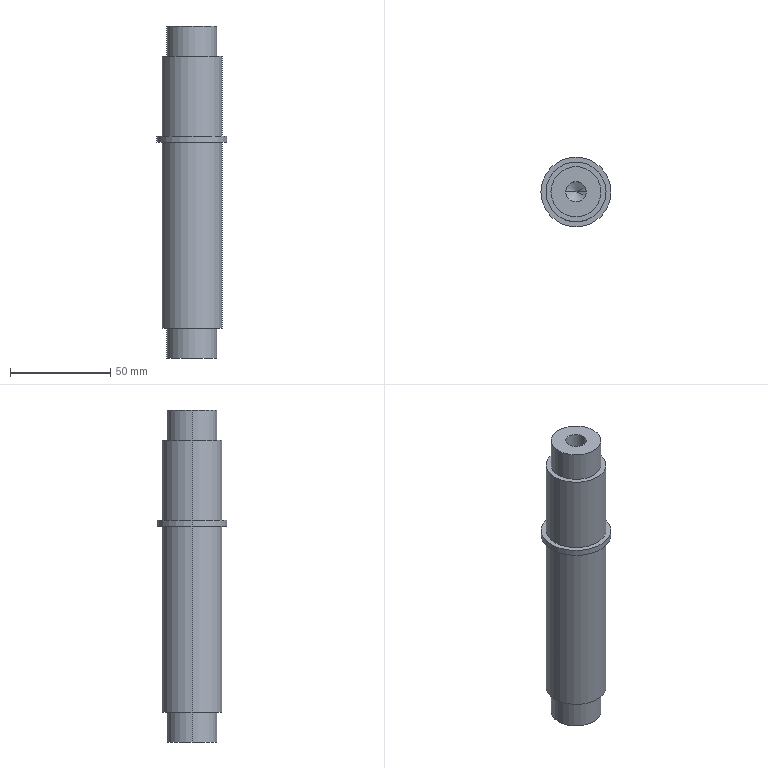Part | SolidWorks | features HoleWzd 2, ICE 2, Extrusion 1, MirrorPattern 1 | 1 solid | 24 faces | box 35 x 35 x 166 mm | volume 106106 mm3 | cylinder 14 | plane 6 | cone 4 | commonest cylinder face diameters 10.2 x4 25 x4 30 x4 35 x2
STEP:
#1=CARTESIAN_POINT('',(-5.1,0.,50.25));
#2=VERTEX_POINT('',#1);
#3=CARTESIAN_POINT('',(5.1,0.,50.25));
#4=VERTEX_POINT('',#3);
#5=CARTESIAN_POINT('',(0.,0.,50.25));
#6=DIRECTION('',(0.,0.,1.));
#7=DIRECTION('',(1.,0.,0.));
#8=AXIS2_PLACEMENT_3D('',#5,#6,#7);
#9=CIRCLE('',#8,5.1);
#10=EDGE_CURVE('',#2,#4,#9,.T.);
#11=ORIENTED_EDGE('',*,*,#10,.F.);
#12=CARTESIAN_POINT('',(-5.1,0.,83.));
#13=VERTEX_POINT('',#12);
#14=CARTESIAN_POINT('',(-5.1,0.,83.));
#15=DIRECTION('',(0.,0.,1.));
#16=VECTOR('',#15,1000.);
#17=LINE('',#14,#16);
#18=EDGE_CURVE('',#2,#13,#17,.T.);
#19=ORIENTED_EDGE('',*,*,#18,.T.);
#20=CARTESIAN_POINT('',(5.1,0.,83.));
#21=VERTEX_POINT('',#20);
#22=CARTESIAN_POINT('',(0.,0.,83.));
#23=DIRECTION('',(0.,0.,1.));
#24=DIRECTION('',(1.,0.,0.));
#25=AXIS2_PLACEMENT_3D('',#22,#23,#24);
#26=CIRCLE('',#25,5.1);
#27=EDGE_CURVE('',#13,#21,#26,.T.);
#28=ORIENTED_EDGE('',*,*,#27,.T.);
#29=CARTESIAN_POINT('',(5.1,0.,83.));
#30=DIRECTION('',(0.,0.,1.));
#31=VECTOR('',#30,1000.);
#32=LINE('',#29,#31);
#33=EDGE_CURVE('',#4,#21,#32,.T.);
#34=ORIENTED_EDGE('',*,*,#33,.F.);
#35=EDGE_LOOP('',(#11,#19,#28,#34));
#36=FACE_OUTER_BOUND('',#35,.T.);
#37=CARTESIAN_POINT('',(0.,0.,83.));
#38=DIRECTION('',(0.,0.,1.));
#39=DIRECTION('',(1.,0.,0.));
#40=AXIS2_PLACEMENT_3D('',#37,#38,#39);
#41=CYLINDRICAL_SURFACE('',#40,5.1);
#42=ADVANCED_FACE('',(#36),#41,.F.);
#43=CARTESIAN_POINT('',(0.,0.,47.186));
#44=VERTEX_POINT('',#43);
#45=CARTESIAN_POINT('',(5.1,0.,50.25));
#46=DIRECTION('',(0.8572,0.,0.515));
#47=VECTOR('',#46,1000.);
#48=LINE('',#45,#47);
#49=EDGE_CURVE('',#44,#4,#48,.T.);
#50=ORIENTED_EDGE('',*,*,#49,.F.);
#51=CARTESIAN_POINT('',(-5.1,0.,50.25));
#52=DIRECTION('',(-0.8572,0.,0.515));
#53=VECTOR('',#52,1000.);
#54=LINE('',#51,#53);
#55=EDGE_CURVE('',#44,#2,#54,.T.);
#56=ORIENTED_EDGE('',*,*,#55,.T.);
#57=ORIENTED_EDGE('',*,*,#10,.T.);
#58=EDGE_LOOP('',(#50,#56,#57));
#59=FACE_OUTER_BOUND('',#58,.T.);
#60=CARTESIAN_POINT('',(0.,0.,50.25));
#61=DIRECTION('',(0.,0.,1.));
#62=DIRECTION('',(1.,0.,0.));
#63=AXIS2_PLACEMENT_3D('',#60,#61,#62);
#64=CONICAL_SURFACE('',#63,5.1,1.03);
#65=ADVANCED_FACE('',(#59),#64,.F.);
#66=CARTESIAN_POINT('',(5.1,0.,-50.25));
#67=VERTEX_POINT('',#66);
#68=CARTESIAN_POINT('',(-5.1,0.,-50.25));
#69=VERTEX_POINT('',#68);
#70=CARTESIAN_POINT('',(0.,0.,-50.25));
#71=DIRECTION('',(0.,0.,-1.));
#72=DIRECTION('',(-1.,0.,0.));
#73=AXIS2_PLACEMENT_3D('',#70,#71,#72);
#74=CIRCLE('',#73,5.1);
#75=EDGE_CURVE('',#67,#69,#74,.T.);
#76=ORIENTED_EDGE('',*,*,#75,.F.);
#77=CARTESIAN_POINT('',(5.1,0.,-83.));
#78=VERTEX_POINT('',#77);
#79=CARTESIAN_POINT('',(5.1,0.,-83.));
#80=DIRECTION('',(0.,0.,-1.));
#81=VECTOR('',#80,1000.);
#82=LINE('',#79,#81);
#83=EDGE_CURVE('',#67,#78,#82,.T.);
#84=ORIENTED_EDGE('',*,*,#83,.T.);
#85=CARTESIAN_POINT('',(-5.1,0.,-83.));
#86=VERTEX_POINT('',#85);
#87=CARTESIAN_POINT('',(0.,0.,-83.));
#88=DIRECTION('',(0.,0.,-1.));
#89=DIRECTION('',(-1.,0.,0.));
#90=AXIS2_PLACEMENT_3D('',#87,#88,#89);
#91=CIRCLE('',#90,5.1);
#92=EDGE_CURVE('',#78,#86,#91,.T.);
#93=ORIENTED_EDGE('',*,*,#92,.T.);
#94=CARTESIAN_POINT('',(-5.1,0.,-83.));
#95=DIRECTION('',(0.,0.,-1.));
#96=VECTOR('',#95,1000.);
#97=LINE('',#94,#96);
#98=EDGE_CURVE('',#69,#86,#97,.T.);
#99=ORIENTED_EDGE('',*,*,#98,.F.);
#100=EDGE_LOOP('',(#76,#84,#93,#99));
#101=FACE_OUTER_BOUND('',#100,.T.);
#102=CARTESIAN_POINT('',(0.,0.,-83.));
#103=DIRECTION('',(0.,0.,-1.));
#104=DIRECTION('',(-1.,0.,0.));
#105=AXIS2_PLACEMENT_3D('',#102,#103,#104);
#106=CYLINDRICAL_SURFACE('',#105,5.1);
#107=ADVANCED_FACE('',(#101),#106,.F.);
#108=CARTESIAN_POINT('',(0.,0.,-47.186));
#109=VERTEX_POINT('',#108);
#110=CARTESIAN_POINT('',(-5.1,0.,-50.25));
#111=DIRECTION('',(-0.8572,0.,-0.515));
#112=VECTOR('',#111,1000.);
#113=LINE('',#110,#112);
#114=EDGE_CURVE('',#109,#69,#113,.T.);
#115=ORIENTED_EDGE('',*,*,#114,.F.);
#116=CARTESIAN_POINT('',(5.1,0.,-50.25));
#117=DIRECTION('',(0.8572,0.,-0.515));
#118=VECTOR('',#117,1000.);
#119=LINE('',#116,#118);
#120=EDGE_CURVE('',#109,#67,#119,.T.);
#121=ORIENTED_EDGE('',*,*,#120,.T.);
#122=ORIENTED_EDGE('',*,*,#75,.T.);
#123=EDGE_LOOP('',(#115,#121,#122));
#124=FACE_OUTER_BOUND('',#123,.T.);
#125=CARTESIAN_POINT('',(0.,0.,-50.25));
#126=DIRECTION('',(0.,0.,-1.));
#127=DIRECTION('',(-1.,0.,0.));
#128=AXIS2_PLACEMENT_3D('',#125,#126,#127);
#129=CONICAL_SURFACE('',#128,5.1,1.03);
#130=ADVANCED_FACE('',(#124),#129,.F.);
#131=CARTESIAN_POINT('',(15.,0.,25.));
#132=VERTEX_POINT('',#131);
#133=CARTESIAN_POINT('',(-15.,0.,25.));
#134=VERTEX_POINT('',#133);
#135=CARTESIAN_POINT('',(0.,0.,25.));
#136=DIRECTION('',(0.,0.,1.));
#137=DIRECTION('',(1.,0.,0.));
#138=AXIS2_PLACEMENT_3D('',#135,#136,#137);
#139=CIRCLE('',#138,15.);
#140=EDGE_CURVE('',#132,#134,#139,.T.);
#141=ORIENTED_EDGE('',*,*,#140,.F.);
#142=CARTESIAN_POINT('',(15.,0.,-68.));
#143=VERTEX_POINT('',#142);
#144=CARTESIAN_POINT('',(15.,0.,68.));
#145=DIRECTION('',(0.,0.,-1.));
#146=VECTOR('',#145,1000.);
#147=LINE('',#144,#146);
#148=EDGE_CURVE('',#132,#143,#147,.T.);
#149=ORIENTED_EDGE('',*,*,#148,.T.);
#150=CARTESIAN_POINT('',(-15.,0.,-68.));
#151=VERTEX_POINT('',#150);
#152=CARTESIAN_POINT('',(0.,0.,-68.));
#153=DIRECTION('',(0.,0.,1.));
#154=DIRECTION('',(1.,0.,0.));
#155=AXIS2_PLACEMENT_3D('',#152,#153,#154);
#156=CIRCLE('',#155,15.);
#157=EDGE_CURVE('',#143,#151,#156,.T.);
#158=ORIENTED_EDGE('',*,*,#157,.T.);
#159=CARTESIAN_POINT('',(-15.,0.,68.));
#160=DIRECTION('',(0.,0.,-1.));
#161=VECTOR('',#160,1000.);
#162=LINE('',#159,#161);
#163=EDGE_CURVE('',#134,#151,#162,.T.);
#164=ORIENTED_EDGE('',*,*,#163,.F.);
#165=EDGE_LOOP('',(#141,#149,#158,#164));
#166=FACE_OUTER_BOUND('',#165,.T.);
#167=CARTESIAN_POINT('',(0.,0.,68.));
#168=DIRECTION('',(0.,0.,-1.));
#169=DIRECTION('',(-1.,0.,0.));
#170=AXIS2_PLACEMENT_3D('',#167,#168,#169);
#171=CYLINDRICAL_SURFACE('',#170,15.);
#172=ADVANCED_FACE('',(#166),#171,.T.);
#173=CARTESIAN_POINT('',(12.5,0.,-83.));
#174=VERTEX_POINT('',#173);
#175=CARTESIAN_POINT('',(-12.5,0.,-83.));
#176=VERTEX_POINT('',#175);
#177=CARTESIAN_POINT('',(0.,0.,-83.));
#178=DIRECTION('',(0.,0.,1.));
#179=DIRECTION('',(1.,0.,0.));
#180=AXIS2_PLACEMENT_3D('',#177,#178,#179);
#181=CIRCLE('',#180,12.5);
#182=EDGE_CURVE('',#174,#176,#181,.T.);
#183=ORIENTED_EDGE('',*,*,#182,.T.);
#184=CARTESIAN_POINT('',(-12.5,0.,-68.));
#185=VERTEX_POINT('',#184);
#186=CARTESIAN_POINT('',(-12.5,0.,-83.));
#187=DIRECTION('',(0.,0.,1.));
#188=VECTOR('',#187,1000.);
#189=LINE('',#186,#188);
#190=EDGE_CURVE('',#176,#185,#189,.T.);
#191=ORIENTED_EDGE('',*,*,#190,.T.);
#192=CARTESIAN_POINT('',(12.5,0.,-68.));
#193=VERTEX_POINT('',#192);
#194=CARTESIAN_POINT('',(0.,0.,-68.));
#195=DIRECTION('',(0.,0.,1.));
#196=DIRECTION('',(1.,0.,0.));
#197=AXIS2_PLACEMENT_3D('',#194,#195,#196);
#198=CIRCLE('',#197,12.5);
#199=EDGE_CURVE('',#193,#185,#198,.T.);
#200=ORIENTED_EDGE('',*,*,#199,.F.);
#201=CARTESIAN_POINT('',(12.5,0.,-83.));
#202=DIRECTION('',(0.,0.,1.));
#203=VECTOR('',#202,1000.);
#204=LINE('',#201,#203);
#205=EDGE_CURVE('',#174,#193,#204,.T.);
#206=ORIENTED_EDGE('',*,*,#205,.F.);
#207=EDGE_LOOP('',(#183,#191,#200,#206));
#208=FACE_OUTER_BOUND('',#207,.T.);
#209=CARTESIAN_POINT('',(0.,0.,-83.));
#210=DIRECTION('',(0.,0.,1.));
#211=DIRECTION('',(1.,0.,0.));
#212=AXIS2_PLACEMENT_3D('',#209,#210,#211);
#213=CYLINDRICAL_SURFACE('',#212,12.5);
#214=ADVANCED_FACE('',(#208),#213,.T.);
#215=CARTESIAN_POINT('',(17.5,0.,28.));
#216=VERTEX_POINT('',#215);
#217=CARTESIAN_POINT('',(-17.5,0.,28.));
#218=VERTEX_POINT('',#217);
#219=CARTESIAN_POINT('',(0.,0.,28.));
#220=DIRECTION('',(0.,0.,1.));
#221=DIRECTION('',(1.,0.,0.));
#222=AXIS2_PLACEMENT_3D('',#219,#220,#221);
#223=CIRCLE('',#222,17.5);
#224=EDGE_CURVE('',#216,#218,#223,.T.);
#225=ORIENTED_EDGE('',*,*,#224,.F.);
#226=CARTESIAN_POINT('',(17.5,0.,25.));
#227=VERTEX_POINT('',#226);
#228=CARTESIAN_POINT('',(17.5,0.,28.));
#229=DIRECTION('',(0.,0.,-1.));
#230=VECTOR('',#229,1000.);
#231=LINE('',#228,#230);
#232=EDGE_CURVE('',#216,#227,#231,.T.);
#233=ORIENTED_EDGE('',*,*,#232,.T.);
#234=CARTESIAN_POINT('',(-17.5,0.,25.));
#235=VERTEX_POINT('',#234);
#236=CARTESIAN_POINT('',(0.,0.,25.));
#237=DIRECTION('',(0.,0.,1.));
#238=DIRECTION('',(1.,0.,0.));
#239=AXIS2_PLACEMENT_3D('',#236,#237,#238);
#240=CIRCLE('',#239,17.5);
#241=EDGE_CURVE('',#227,#235,#240,.T.);
#242=ORIENTED_EDGE('',*,*,#241,.T.);
#243=CARTESIAN_POINT('',(-17.5,0.,28.));
#244=DIRECTION('',(0.,0.,-1.));
#245=VECTOR('',#244,1000.);
#246=LINE('',#243,#245);
#247=EDGE_CURVE('',#218,#235,#246,.T.);
#248=ORIENTED_EDGE('',*,*,#247,.F.);
#249=EDGE_LOOP('',(#225,#233,#242,#248));
#250=FACE_OUTER_BOUND('',#249,.T.);
#251=CARTESIAN_POINT('',(0.,0.,28.));
#252=DIRECTION('',(0.,0.,-1.));
#253=DIRECTION('',(-1.,0.,0.));
#254=AXIS2_PLACEMENT_3D('',#251,#252,#253);
#255=CYLINDRICAL_SURFACE('',#254,17.5);
#256=ADVANCED_FACE('',(#250),#255,.T.);
#257=CARTESIAN_POINT('',(12.5,0.,83.));
#258=VERTEX_POINT('',#257);
#259=CARTESIAN_POINT('',(-12.5,0.,83.));
#260=VERTEX_POINT('',#259);
#261=CARTESIAN_POINT('',(0.,0.,83.));
#262=DIRECTION('',(0.,0.,1.));
#263=DIRECTION('',(1.,0.,0.));
#264=AXIS2_PLACEMENT_3D('',#261,#262,#263);
#265=CIRCLE('',#264,12.5);
#266=EDGE_CURVE('',#258,#260,#265,.T.);
#267=ORIENTED_EDGE('',*,*,#266,.F.);
#268=CARTESIAN_POINT('',(12.5,0.,68.));
#269=VERTEX_POINT('',#268);
#270=CARTESIAN_POINT('',(12.5,0.,83.));
#271=DIRECTION('',(0.,0.,-1.));
#272=VECTOR('',#271,1000.);
#273=LINE('',#270,#272);
#274=EDGE_CURVE('',#258,#269,#273,.T.);
#275=ORIENTED_EDGE('',*,*,#274,.T.);
#276=CARTESIAN_POINT('',(-12.5,0.,68.));
#277=VERTEX_POINT('',#276);
#278=CARTESIAN_POINT('',(0.,0.,68.));
#279=DIRECTION('',(0.,0.,1.));
#280=DIRECTION('',(1.,0.,0.));
#281=AXIS2_PLACEMENT_3D('',#278,#279,#280);
#282=CIRCLE('',#281,12.5);
#283=EDGE_CURVE('',#269,#277,#282,.T.);
#284=ORIENTED_EDGE('',*,*,#283,.T.);
#285=CARTESIAN_POINT('',(-12.5,0.,83.));
#286=DIRECTION('',(0.,0.,-1.));
#287=VECTOR('',#286,1000.);
#288=LINE('',#285,#287);
#289=EDGE_CURVE('',#260,#277,#288,.T.);
#290=ORIENTED_EDGE('',*,*,#289,.F.);
#291=EDGE_LOOP('',(#267,#275,#284,#290));
#292=FACE_OUTER_BOUND('',#291,.T.);
#293=CARTESIAN_POINT('',(0.,0.,83.));
#294=DIRECTION('',(0.,0.,-1.));
#295=DIRECTION('',(-1.,0.,0.));
#296=AXIS2_PLACEMENT_3D('',#293,#294,#295);
#297=CYLINDRICAL_SURFACE('',#296,12.5);
#298=ADVANCED_FACE('',(#292),#297,.T.);
#299=CARTESIAN_POINT('',(15.,0.,68.));
#300=VERTEX_POINT('',#299);
#301=CARTESIAN_POINT('',(-15.,0.,68.));
#302=VERTEX_POINT('',#301);
#303=CARTESIAN_POINT('',(0.,0.,68.));
#304=DIRECTION('',(0.,0.,1.));
#305=DIRECTION('',(1.,0.,0.));
#306=AXIS2_PLACEMENT_3D('',#303,#304,#305);
#307=CIRCLE('',#306,15.);
#308=EDGE_CURVE('',#300,#302,#307,.T.);
#309=ORIENTED_EDGE('',*,*,#308,.F.);
#310=CARTESIAN_POINT('',(15.,0.,28.));
#311=VERTEX_POINT('',#310);
#312=CARTESIAN_POINT('',(15.,0.,68.));
#313=DIRECTION('',(0.,0.,-1.));
#314=VECTOR('',#313,1000.);
#315=LINE('',#312,#314);
#316=EDGE_CURVE('',#300,#311,#315,.T.);
#317=ORIENTED_EDGE('',*,*,#316,.T.);
#318=CARTESIAN_POINT('',(-15.,0.,28.));
#319=VERTEX_POINT('',#318);
#320=CARTESIAN_POINT('',(0.,0.,28.));
#321=DIRECTION('',(0.,0.,1.));
#322=DIRECTION('',(1.,0.,0.));
#323=AXIS2_PLACEMENT_3D('',#320,#321,#322);
#324=CIRCLE('',#323,15.);
#325=EDGE_CURVE('',#311,#319,#324,.T.);
#326=ORIENTED_EDGE('',*,*,#325,.T.);
#327=CARTESIAN_POINT('',(-15.,0.,68.));
#328=DIRECTION('',(0.,0.,-1.));
#329=VECTOR('',#328,1000.);
#330=LINE('',#327,#329);
#331=EDGE_CURVE('',#302,#319,#330,.T.);
#332=ORIENTED_EDGE('',*,*,#331,.F.);
#333=EDGE_LOOP('',(#309,#317,#326,#332));
#334=FACE_OUTER_BOUND('',#333,.T.);
#335=CARTESIAN_POINT('',(0.,0.,68.));
#336=DIRECTION('',(0.,0.,-1.));
#337=DIRECTION('',(-1.,0.,0.));
#338=AXIS2_PLACEMENT_3D('',#335,#336,#337);
#339=CYLINDRICAL_SURFACE('',#338,15.);
#340=ADVANCED_FACE('',(#334),#339,.T.);
#341=CARTESIAN_POINT('',(0.,0.,68.));
#342=DIRECTION('',(0.,0.,1.));
#343=DIRECTION('',(1.,0.,0.));
#344=AXIS2_PLACEMENT_3D('',#341,#342,#343);
#345=CIRCLE('',#344,15.);
#346=EDGE_CURVE('',#302,#300,#345,.T.);
#347=ORIENTED_EDGE('',*,*,#346,.T.);
#348=ORIENTED_EDGE('',*,*,#308,.T.);
#349=EDGE_LOOP('',(#347,#348));
#350=FACE_OUTER_BOUND('',#349,.T.);
#351=CARTESIAN_POINT('',(0.,0.,68.));
#352=DIRECTION('',(0.,0.,1.));
#353=DIRECTION('',(1.,0.,0.));
#354=AXIS2_PLACEMENT_3D('',#351,#352,#353);
#355=CIRCLE('',#354,12.5);
#356=EDGE_CURVE('',#277,#269,#355,.T.);
#357=ORIENTED_EDGE('',*,*,#356,.F.);
#358=ORIENTED_EDGE('',*,*,#283,.F.);
#359=EDGE_LOOP('',(#357,#358));
#360=FACE_BOUND('',#359,.T.);
#361=CARTESIAN_POINT('',(0.,0.,68.));
#362=DIRECTION('',(0.,0.,1.));
#363=DIRECTION('',(1.,0.,0.));
#364=AXIS2_PLACEMENT_3D('',#361,#362,#363);
#365=PLANE('',#364);
#366=ADVANCED_FACE('',(#350,#360),#365,.T.);
#367=ORIENTED_EDGE('',*,*,#316,.F.);
#368=ORIENTED_EDGE('',*,*,#346,.F.);
#369=ORIENTED_EDGE('',*,*,#331,.T.);
#370=CARTESIAN_POINT('',(0.,0.,28.));
#371=DIRECTION('',(0.,0.,1.));
#372=DIRECTION('',(1.,0.,0.));
#373=AXIS2_PLACEMENT_3D('',#370,#371,#372);
#374=CIRCLE('',#373,15.);
#375=EDGE_CURVE('',#319,#311,#374,.T.);
#376=ORIENTED_EDGE('',*,*,#375,.T.);
#377=EDGE_LOOP('',(#367,#368,#369,#376));
#378=FACE_OUTER_BOUND('',#377,.T.);
#379=CARTESIAN_POINT('',(0.,0.,68.));
#380=DIRECTION('',(0.,0.,-1.));
#381=DIRECTION('',(-1.,0.,0.));
#382=AXIS2_PLACEMENT_3D('',#379,#380,#381);
#383=CYLINDRICAL_SURFACE('',#382,15.);
#384=ADVANCED_FACE('',(#378),#383,.T.);
#385=ORIENTED_EDGE('',*,*,#274,.F.);
#386=CARTESIAN_POINT('',(0.,0.,83.));
#387=DIRECTION('',(0.,0.,1.));
#388=DIRECTION('',(1.,0.,0.));
#389=AXIS2_PLACEMENT_3D('',#386,#387,#388);
#390=CIRCLE('',#389,12.5);
#391=EDGE_CURVE('',#260,#258,#390,.T.);
#392=ORIENTED_EDGE('',*,*,#391,.F.);
#393=ORIENTED_EDGE('',*,*,#289,.T.);
#394=ORIENTED_EDGE('',*,*,#356,.T.);
#395=EDGE_LOOP('',(#385,#392,#393,#394));
#396=FACE_OUTER_BOUND('',#395,.T.);
#397=CARTESIAN_POINT('',(0.,0.,83.));
#398=DIRECTION('',(0.,0.,-1.));
#399=DIRECTION('',(-1.,0.,0.));
#400=AXIS2_PLACEMENT_3D('',#397,#398,#399);
#401=CYLINDRICAL_SURFACE('',#400,12.5);
#402=ADVANCED_FACE('',(#396),#401,.T.);
#403=CARTESIAN_POINT('',(0.,0.,83.));
#404=DIRECTION('',(0.,0.,1.));
#405=DIRECTION('',(1.,0.,0.));
#406=AXIS2_PLACEMENT_3D('',#403,#404,#405);
#407=CIRCLE('',#406,5.1);
#408=EDGE_CURVE('',#21,#13,#407,.T.);
#409=ORIENTED_EDGE('',*,*,#408,.F.);
#410=ORIENTED_EDGE('',*,*,#27,.F.);
#411=EDGE_LOOP('',(#409,#410));
#412=FACE_BOUND('',#411,.T.);
#413=ORIENTED_EDGE('',*,*,#391,.T.);
#414=ORIENTED_EDGE('',*,*,#266,.T.);
#415=EDGE_LOOP('',(#413,#414));
#416=FACE_OUTER_BOUND('',#415,.T.);
#417=CARTESIAN_POINT('',(0.,0.,83.));
#418=DIRECTION('',(0.,0.,1.));
#419=DIRECTION('',(1.,0.,0.));
#420=AXIS2_PLACEMENT_3D('',#417,#418,#419);
#421=PLANE('',#420);
#422=ADVANCED_FACE('',(#412,#416),#421,.T.);
#423=CARTESIAN_POINT('',(0.,0.,28.));
#424=DIRECTION('',(0.,0.,1.));
#425=DIRECTION('',(1.,0.,0.));
#426=AXIS2_PLACEMENT_3D('',#423,#424,#425);
#427=CIRCLE('',#426,17.5);
#428=EDGE_CURVE('',#218,#216,#427,.T.);
#429=ORIENTED_EDGE('',*,*,#428,.T.);
#430=ORIENTED_EDGE('',*,*,#224,.T.);
#431=EDGE_LOOP('',(#429,#430));
#432=FACE_OUTER_BOUND('',#431,.T.);
#433=ORIENTED_EDGE('',*,*,#375,.F.);
#434=ORIENTED_EDGE('',*,*,#325,.F.);
#435=EDGE_LOOP('',(#433,#434));
#436=FACE_BOUND('',#435,.T.);
#437=CARTESIAN_POINT('',(0.,0.,28.));
#438=DIRECTION('',(0.,0.,1.));
#439=DIRECTION('',(1.,0.,0.));
#440=AXIS2_PLACEMENT_3D('',#437,#438,#439);
#441=PLANE('',#440);
#442=ADVANCED_FACE('',(#432,#436),#441,.T.);
#443=CARTESIAN_POINT('',(0.,0.,25.));
#444=DIRECTION('',(0.,0.,1.));
#445=DIRECTION('',(1.,0.,0.));
#446=AXIS2_PLACEMENT_3D('',#443,#444,#445);
#447=CIRCLE('',#446,17.5);
#448=EDGE_CURVE('',#235,#227,#447,.T.);
#449=ORIENTED_EDGE('',*,*,#448,.F.);
#450=ORIENTED_EDGE('',*,*,#241,.F.);
#451=EDGE_LOOP('',(#449,#450));
#452=FACE_OUTER_BOUND('',#451,.T.);
#453=CARTESIAN_POINT('',(0.,0.,25.));
#454=DIRECTION('',(0.,0.,1.));
#455=DIRECTION('',(1.,0.,0.));
#456=AXIS2_PLACEMENT_3D('',#453,#454,#455);
#457=CIRCLE('',#456,15.);
#458=EDGE_CURVE('',#134,#132,#457,.T.);
#459=ORIENTED_EDGE('',*,*,#458,.T.);
#460=ORIENTED_EDGE('',*,*,#140,.T.);
#461=EDGE_LOOP('',(#459,#460));
#462=FACE_BOUND('',#461,.T.);
#463=CARTESIAN_POINT('',(0.,0.,25.));
#464=DIRECTION('',(0.,0.,1.));
#465=DIRECTION('',(1.,0.,0.));
#466=AXIS2_PLACEMENT_3D('',#463,#464,#465);
#467=PLANE('',#466);
#468=ADVANCED_FACE('',(#452,#462),#467,.F.);
#469=ORIENTED_EDGE('',*,*,#232,.F.);
#470=ORIENTED_EDGE('',*,*,#428,.F.);
#471=ORIENTED_EDGE('',*,*,#247,.T.);
#472=ORIENTED_EDGE('',*,*,#448,.T.);
#473=EDGE_LOOP('',(#469,#470,#471,#472));
#474=FACE_OUTER_BOUND('',#473,.T.);
#475=CARTESIAN_POINT('',(0.,0.,28.));
#476=DIRECTION('',(0.,0.,-1.));
#477=DIRECTION('',(-1.,0.,0.));
#478=AXIS2_PLACEMENT_3D('',#475,#476,#477);
#479=CYLINDRICAL_SURFACE('',#478,17.5);
#480=ADVANCED_FACE('',(#474),#479,.T.);
#481=CARTESIAN_POINT('',(0.,0.,-83.));
#482=DIRECTION('',(0.,0.,-1.));
#483=DIRECTION('',(-1.,0.,0.));
#484=AXIS2_PLACEMENT_3D('',#481,#482,#483);
#485=CIRCLE('',#484,5.1);
#486=EDGE_CURVE('',#86,#78,#485,.T.);
#487=ORIENTED_EDGE('',*,*,#486,.F.);
#488=ORIENTED_EDGE('',*,*,#92,.F.);
#489=EDGE_LOOP('',(#487,#488));
#490=FACE_BOUND('',#489,.T.);
#491=ORIENTED_EDGE('',*,*,#182,.F.);
#492=CARTESIAN_POINT('',(0.,0.,-83.));
#493=DIRECTION('',(0.,0.,1.));
#494=DIRECTION('',(1.,0.,0.));
#495=AXIS2_PLACEMENT_3D('',#492,#493,#494);
#496=CIRCLE('',#495,12.5);
#497=EDGE_CURVE('',#176,#174,#496,.T.);
#498=ORIENTED_EDGE('',*,*,#497,.F.);
#499=EDGE_LOOP('',(#491,#498));
#500=FACE_OUTER_BOUND('',#499,.T.);
#501=CARTESIAN_POINT('',(0.,0.,-83.));
#502=DIRECTION('',(0.,0.,-1.));
#503=DIRECTION('',(1.,0.,0.));
#504=AXIS2_PLACEMENT_3D('',#501,#502,#503);
#505=PLANE('',#504);
#506=ADVANCED_FACE('',(#490,#500),#505,.T.);
#507=ORIENTED_EDGE('',*,*,#190,.F.);
#508=ORIENTED_EDGE('',*,*,#497,.T.);
#509=ORIENTED_EDGE('',*,*,#205,.T.);
#510=CARTESIAN_POINT('',(0.,0.,-68.));
#511=DIRECTION('',(0.,0.,1.));
#512=DIRECTION('',(1.,0.,0.));
#513=AXIS2_PLACEMENT_3D('',#510,#511,#512);
#514=CIRCLE('',#513,12.5);
#515=EDGE_CURVE('',#185,#193,#514,.T.);
#516=ORIENTED_EDGE('',*,*,#515,.F.);
#517=EDGE_LOOP('',(#507,#508,#509,#516));
#518=FACE_OUTER_BOUND('',#517,.T.);
#519=CARTESIAN_POINT('',(0.,0.,-83.));
#520=DIRECTION('',(0.,0.,1.));
#521=DIRECTION('',(1.,0.,0.));
#522=AXIS2_PLACEMENT_3D('',#519,#520,#521);
#523=CYLINDRICAL_SURFACE('',#522,12.5);
#524=ADVANCED_FACE('',(#518),#523,.T.);
#525=ORIENTED_EDGE('',*,*,#199,.T.);
#526=ORIENTED_EDGE('',*,*,#515,.T.);
#527=EDGE_LOOP('',(#525,#526));
#528=FACE_BOUND('',#527,.T.);
#529=CARTESIAN_POINT('',(0.,0.,-68.));
#530=DIRECTION('',(0.,0.,1.));
#531=DIRECTION('',(1.,0.,0.));
#532=AXIS2_PLACEMENT_3D('',#529,#530,#531);
#533=CIRCLE('',#532,15.);
#534=EDGE_CURVE('',#151,#143,#533,.T.);
#535=ORIENTED_EDGE('',*,*,#534,.F.);
#536=ORIENTED_EDGE('',*,*,#157,.F.);
#537=EDGE_LOOP('',(#535,#536));
#538=FACE_OUTER_BOUND('',#537,.T.);
#539=CARTESIAN_POINT('',(0.,0.,-68.));
#540=DIRECTION('',(0.,0.,1.));
#541=DIRECTION('',(1.,0.,0.));
#542=AXIS2_PLACEMENT_3D('',#539,#540,#541);
#543=PLANE('',#542);
#544=ADVANCED_FACE('',(#528,#538),#543,.F.);
#545=ORIENTED_EDGE('',*,*,#148,.F.);
#546=ORIENTED_EDGE('',*,*,#458,.F.);
#547=ORIENTED_EDGE('',*,*,#163,.T.);
#548=ORIENTED_EDGE('',*,*,#534,.T.);
#549=EDGE_LOOP('',(#545,#546,#547,#548));
#550=FACE_OUTER_BOUND('',#549,.T.);
#551=CARTESIAN_POINT('',(0.,0.,68.));
#552=DIRECTION('',(0.,0.,-1.));
#553=DIRECTION('',(-1.,0.,0.));
#554=AXIS2_PLACEMENT_3D('',#551,#552,#553);
#555=CYLINDRICAL_SURFACE('',#554,15.);
#556=ADVANCED_FACE('',(#550),#555,.T.);
#557=ORIENTED_EDGE('',*,*,#120,.F.);
#558=ORIENTED_EDGE('',*,*,#114,.T.);
#559=CARTESIAN_POINT('',(0.,0.,-50.25));
#560=DIRECTION('',(0.,0.,-1.));
#561=DIRECTION('',(-1.,0.,0.));
#562=AXIS2_PLACEMENT_3D('',#559,#560,#561);
#563=CIRCLE('',#562,5.1);
#564=EDGE_CURVE('',#69,#67,#563,.T.);
#565=ORIENTED_EDGE('',*,*,#564,.T.);
#566=EDGE_LOOP('',(#557,#558,#565));
#567=FACE_OUTER_BOUND('',#566,.T.);
#568=CARTESIAN_POINT('',(0.,0.,-50.25));
#569=DIRECTION('',(0.,0.,-1.));
#570=DIRECTION('',(-1.,0.,0.));
#571=AXIS2_PLACEMENT_3D('',#568,#569,#570);
#572=CONICAL_SURFACE('',#571,5.1,1.03);
#573=ADVANCED_FACE('',(#567),#572,.F.);
#574=ORIENTED_EDGE('',*,*,#83,.F.);
#575=ORIENTED_EDGE('',*,*,#564,.F.);
#576=ORIENTED_EDGE('',*,*,#98,.T.);
#577=ORIENTED_EDGE('',*,*,#486,.T.);
#578=EDGE_LOOP('',(#574,#575,#576,#577));
#579=FACE_OUTER_BOUND('',#578,.T.);
#580=CARTESIAN_POINT('',(0.,0.,-83.));
#581=DIRECTION('',(0.,0.,-1.));
#582=DIRECTION('',(-1.,0.,0.));
#583=AXIS2_PLACEMENT_3D('',#580,#581,#582);
#584=CYLINDRICAL_SURFACE('',#583,5.1);
#585=ADVANCED_FACE('',(#579),#584,.F.);
#586=ORIENTED_EDGE('',*,*,#55,.F.);
#587=ORIENTED_EDGE('',*,*,#49,.T.);
#588=CARTESIAN_POINT('',(0.,0.,50.25));
#589=DIRECTION('',(0.,0.,1.));
#590=DIRECTION('',(1.,0.,0.));
#591=AXIS2_PLACEMENT_3D('',#588,#589,#590);
#592=CIRCLE('',#591,5.1);
#593=EDGE_CURVE('',#4,#2,#592,.T.);
#594=ORIENTED_EDGE('',*,*,#593,.T.);
#595=EDGE_LOOP('',(#586,#587,#594));
#596=FACE_OUTER_BOUND('',#595,.T.);
#597=CARTESIAN_POINT('',(0.,0.,50.25));
#598=DIRECTION('',(0.,0.,1.));
#599=DIRECTION('',(1.,0.,0.));
#600=AXIS2_PLACEMENT_3D('',#597,#598,#599);
#601=CONICAL_SURFACE('',#600,5.1,1.03);
#602=ADVANCED_FACE('',(#596),#601,.F.);
#603=ORIENTED_EDGE('',*,*,#18,.F.);
#604=ORIENTED_EDGE('',*,*,#593,.F.);
#605=ORIENTED_EDGE('',*,*,#33,.T.);
#606=ORIENTED_EDGE('',*,*,#408,.T.);
#607=EDGE_LOOP('',(#603,#604,#605,#606));
#608=FACE_OUTER_BOUND('',#607,.T.);
#609=CARTESIAN_POINT('',(0.,0.,83.));
#610=DIRECTION('',(0.,0.,1.));
#611=DIRECTION('',(1.,0.,0.));
#612=AXIS2_PLACEMENT_3D('',#609,#610,#611);
#613=CYLINDRICAL_SURFACE('',#612,5.1);
#614=ADVANCED_FACE('',(#608),#613,.F.);
#615=CLOSED_SHELL('',(#42,#65,#107,#130,#172,#214,#256,#298,#340,#366,#384,#402,#422,#442,#468,#480,#506,#524,#544,#556,#573,#585,#602,#614));
#616=MANIFOLD_SOLID_BREP('',#615);
#617=CARTESIAN_POINT('',(0.,0.,0.));
#618=DIRECTION('',(0.,0.,1.));
#619=DIRECTION('',(1.,0.,0.));
#620=AXIS2_PLACEMENT_3D('',#617,#618,#619);
#621=(LENGTH_UNIT()NAMED_UNIT(*)SI_UNIT(.MILLI.,.METRE.));
#622=UNCERTAINTY_MEASURE_WITH_UNIT(LENGTH_MEASURE(0.00001),#621,'','');
#623=(NAMED_UNIT(*)PLANE_ANGLE_UNIT()SI_UNIT($,.RADIAN.));
#624=(NAMED_UNIT(*)SI_UNIT($,.STERADIAN.)SOLID_ANGLE_UNIT());
#625=(GEOMETRIC_REPRESENTATION_CONTEXT(3)GLOBAL_UNCERTAINTY_ASSIGNED_CONTEXT((#622))GLOBAL_UNIT_ASSIGNED_CONTEXT((#621,#623,#624))REPRESENTATION_CONTEXT('',''));
#626=ADVANCED_BREP_SHAPE_REPRESENTATION('',(#616,#620),#625);